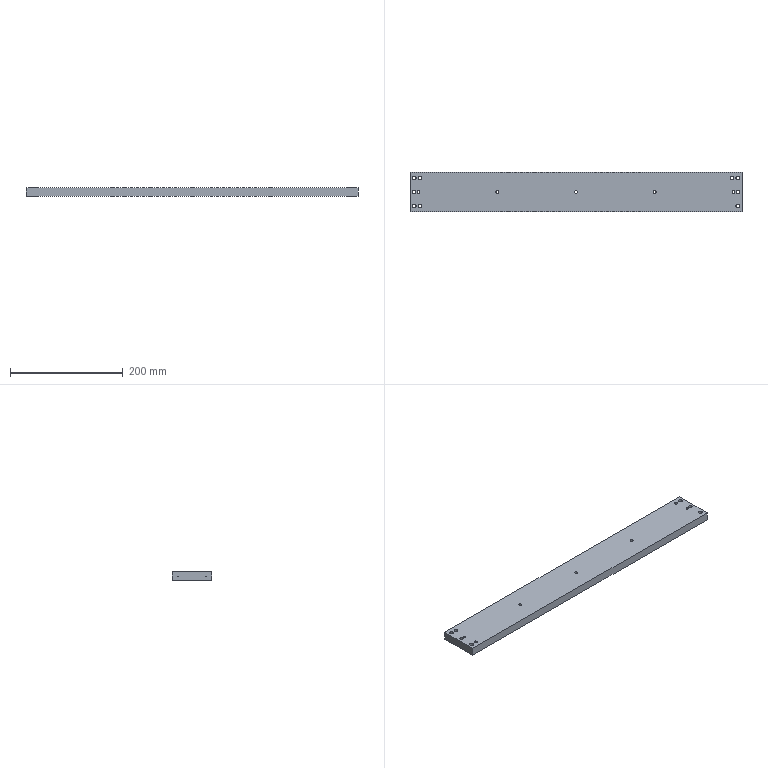Part | NX | 1 solid | 33 faces | box 590 x 70 x 15 mm | volume 612257 mm3 | cylinder 21 | plane 12 | commonest cylinder face diameters 5 x5 6 x5 6.6 x4 11 x4 3.3 x3
STEP:
#1=CARTESIAN_POINT('',(579.9,33.503,3.695));
#2=VERTEX_POINT('',#1);
#3=CARTESIAN_POINT('',(579.9,33.503,2.305));
#4=VERTEX_POINT('',#3);
#5=CARTESIAN_POINT('',(579.9,35.,3.));
#6=DIRECTION('',(1.,0.,0.));
#7=DIRECTION('',(0.,0.,-1.));
#8=AXIS2_PLACEMENT_3D('',#5,#6,#7);
#9=CIRCLE('',#8,1.65);
#10=EDGE_CURVE('',#2,#4,#9,.T.);
#11=ORIENTED_EDGE('',*,*,#10,.F.);
#12=CARTESIAN_POINT('',(579.9,33.503,2.305));
#13=CARTESIAN_POINT('',(580.015,33.304,2.735));
#14=CARTESIAN_POINT('',(580.015,33.304,3.265));
#15=CARTESIAN_POINT('',(579.9,33.503,3.695));
#16=B_SPLINE_CURVE_WITH_KNOTS('',3,(#12,#13,#14,#15),.UNSPECIFIED.,.F.,.F.,(4,4),(0.,0.001444),.UNSPECIFIED.);
#17=EDGE_CURVE('',#4,#2,#16,.T.);
#18=ORIENTED_EDGE('',*,*,#17,.F.);
#19=EDGE_LOOP('',(#11,#18));
#20=FACE_BOUND('',#19,.T.);
#21=CARTESIAN_POINT('',(590.,35.,3.));
#22=DIRECTION('',(1.,0.,0.));
#23=DIRECTION('',(0.,0.,-1.));
#24=AXIS2_PLACEMENT_3D('',#21,#22,#23);
#25=CYLINDRICAL_SURFACE('',#24,1.65);
#26=ADVANCED_FACE('',(#20),#25,.F.);
#27=ORIENTED_EDGE('',*,*,#10,.T.);
#28=CARTESIAN_POINT('',(579.9,33.503,0.));
#29=DIRECTION('',(0.,0.,-1.));
#30=VECTOR('',#29,1000.);
#31=LINE('',#28,#30);
#32=EDGE_CURVE('',#2,#4,#31,.T.);
#33=ORIENTED_EDGE('',*,*,#32,.F.);
#34=EDGE_LOOP('',(#27,#33));
#35=FACE_BOUND('',#34,.T.);
#36=CARTESIAN_POINT('',(579.9,35.,3.));
#37=DIRECTION('',(-1.,0.,0.));
#38=DIRECTION('',(0.,0.,1.));
#39=AXIS2_PLACEMENT_3D('',#36,#37,#38);
#40=PLANE('',#39);
#41=ADVANCED_FACE('',(#35),#40,.F.);
#42=CARTESIAN_POINT('',(579.9,36.497,2.305));
#43=VERTEX_POINT('',#42);
#44=CARTESIAN_POINT('',(579.9,36.497,3.695));
#45=VERTEX_POINT('',#44);
#46=CARTESIAN_POINT('',(579.9,35.,3.));
#47=DIRECTION('',(1.,0.,0.));
#48=DIRECTION('',(0.,0.,-1.));
#49=AXIS2_PLACEMENT_3D('',#46,#47,#48);
#50=CIRCLE('',#49,1.65);
#51=EDGE_CURVE('',#43,#45,#50,.T.);
#52=ORIENTED_EDGE('',*,*,#51,.T.);
#53=CARTESIAN_POINT('',(579.9,36.497,0.));
#54=DIRECTION('',(0.,0.,1.));
#55=VECTOR('',#54,1000.);
#56=LINE('',#53,#55);
#57=EDGE_CURVE('',#43,#45,#56,.T.);
#58=ORIENTED_EDGE('',*,*,#57,.F.);
#59=EDGE_LOOP('',(#52,#58));
#60=FACE_BOUND('',#59,.T.);
#61=CARTESIAN_POINT('',(579.9,35.,3.));
#62=DIRECTION('',(-1.,0.,0.));
#63=DIRECTION('',(0.,0.,1.));
#64=AXIS2_PLACEMENT_3D('',#61,#62,#63);
#65=PLANE('',#64);
#66=ADVANCED_FACE('',(#60),#65,.F.);
#67=ORIENTED_EDGE('',*,*,#51,.F.);
#68=CARTESIAN_POINT('',(579.9,36.497,3.695));
#69=CARTESIAN_POINT('',(580.015,36.696,3.265));
#70=CARTESIAN_POINT('',(580.015,36.696,2.735));
#71=CARTESIAN_POINT('',(579.9,36.497,2.305));
#72=B_SPLINE_CURVE_WITH_KNOTS('',3,(#68,#69,#70,#71),.UNSPECIFIED.,.F.,.F.,(4,4),(0.,0.001444),.UNSPECIFIED.);
#73=EDGE_CURVE('',#45,#43,#72,.T.);
#74=ORIENTED_EDGE('',*,*,#73,.F.);
#75=EDGE_LOOP('',(#67,#74));
#76=FACE_BOUND('',#75,.T.);
#77=CARTESIAN_POINT('',(590.,35.,3.));
#78=DIRECTION('',(1.,0.,0.));
#79=DIRECTION('',(0.,0.,-1.));
#80=AXIS2_PLACEMENT_3D('',#77,#78,#79);
#81=CYLINDRICAL_SURFACE('',#80,1.65);
#82=ADVANCED_FACE('',(#76),#81,.F.);
#83=CARTESIAN_POINT('',(2.,10.,6.4));
#84=VERTEX_POINT('',#83);
#85=CARTESIAN_POINT('',(7.5,10.,6.4));
#86=DIRECTION('',(0.,0.,-1.));
#87=DIRECTION('',(-1.,0.,0.));
#88=AXIS2_PLACEMENT_3D('',#85,#86,#87);
#89=CIRCLE('',#88,5.5);
#90=EDGE_CURVE('',#84,#84,#89,.T.);
#91=ORIENTED_EDGE('',*,*,#90,.T.);
#92=EDGE_LOOP('',(#91));
#93=FACE_BOUND('',#92,.T.);
#94=CARTESIAN_POINT('',(4.2,10.,6.4));
#95=VERTEX_POINT('',#94);
#96=CARTESIAN_POINT('',(7.5,10.,6.4));
#97=DIRECTION('',(0.,0.,-1.));
#98=DIRECTION('',(-1.,0.,0.));
#99=AXIS2_PLACEMENT_3D('',#96,#97,#98);
#100=CIRCLE('',#99,3.3);
#101=EDGE_CURVE('',#95,#95,#100,.T.);
#102=ORIENTED_EDGE('',*,*,#101,.F.);
#103=EDGE_LOOP('',(#102));
#104=FACE_BOUND('',#103,.T.);
#105=CARTESIAN_POINT('',(10.8,10.,6.4));
#106=DIRECTION('',(0.,0.,1.));
#107=DIRECTION('',(1.,0.,0.));
#108=AXIS2_PLACEMENT_3D('',#105,#106,#107);
#109=PLANE('',#108);
#110=ADVANCED_FACE('',(#93,#104),#109,.F.);
#111=CARTESIAN_POINT('',(13.,60.,6.4));
#112=VERTEX_POINT('',#111);
#113=CARTESIAN_POINT('',(7.5,60.,6.4));
#114=DIRECTION('',(0.,0.,-1.));
#115=DIRECTION('',(1.,0.,0.));
#116=AXIS2_PLACEMENT_3D('',#113,#114,#115);
#117=CIRCLE('',#116,5.5);
#118=EDGE_CURVE('',#112,#112,#117,.T.);
#119=ORIENTED_EDGE('',*,*,#118,.T.);
#120=EDGE_LOOP('',(#119));
#121=FACE_BOUND('',#120,.T.);
#122=CARTESIAN_POINT('',(10.8,60.,6.4));
#123=VERTEX_POINT('',#122);
#124=CARTESIAN_POINT('',(7.5,60.,6.4));
#125=DIRECTION('',(0.,0.,-1.));
#126=DIRECTION('',(1.,0.,0.));
#127=AXIS2_PLACEMENT_3D('',#124,#125,#126);
#128=CIRCLE('',#127,3.3);
#129=EDGE_CURVE('',#123,#123,#128,.T.);
#130=ORIENTED_EDGE('',*,*,#129,.F.);
#131=EDGE_LOOP('',(#130));
#132=FACE_BOUND('',#131,.T.);
#133=CARTESIAN_POINT('',(10.8,10.,6.4));
#134=DIRECTION('',(0.,0.,1.));
#135=DIRECTION('',(1.,0.,0.));
#136=AXIS2_PLACEMENT_3D('',#133,#134,#135);
#137=PLANE('',#136);
#138=ADVANCED_FACE('',(#121,#132),#137,.F.);
#139=CARTESIAN_POINT('',(588.,10.,6.4));
#140=VERTEX_POINT('',#139);
#141=CARTESIAN_POINT('',(582.5,10.,6.4));
#142=DIRECTION('',(0.,0.,-1.));
#143=DIRECTION('',(1.,0.,0.));
#144=AXIS2_PLACEMENT_3D('',#141,#142,#143);
#145=CIRCLE('',#144,5.5);
#146=EDGE_CURVE('',#140,#140,#145,.T.);
#147=ORIENTED_EDGE('',*,*,#146,.T.);
#148=EDGE_LOOP('',(#147));
#149=FACE_BOUND('',#148,.T.);
#150=CARTESIAN_POINT('',(585.8,10.,6.4));
#151=VERTEX_POINT('',#150);
#152=CARTESIAN_POINT('',(582.5,10.,6.4));
#153=DIRECTION('',(0.,0.,-1.));
#154=DIRECTION('',(1.,0.,0.));
#155=AXIS2_PLACEMENT_3D('',#152,#153,#154);
#156=CIRCLE('',#155,3.3);
#157=EDGE_CURVE('',#151,#151,#156,.T.);
#158=ORIENTED_EDGE('',*,*,#157,.F.);
#159=EDGE_LOOP('',(#158));
#160=FACE_BOUND('',#159,.T.);
#161=CARTESIAN_POINT('',(10.8,10.,6.4));
#162=DIRECTION('',(0.,0.,1.));
#163=DIRECTION('',(1.,0.,0.));
#164=AXIS2_PLACEMENT_3D('',#161,#162,#163);
#165=PLANE('',#164);
#166=ADVANCED_FACE('',(#149,#160),#165,.F.);
#167=CARTESIAN_POINT('',(588.,60.,6.4));
#168=VERTEX_POINT('',#167);
#169=CARTESIAN_POINT('',(582.5,60.,6.4));
#170=DIRECTION('',(0.,0.,-1.));
#171=DIRECTION('',(1.,0.,0.));
#172=AXIS2_PLACEMENT_3D('',#169,#170,#171);
#173=CIRCLE('',#172,5.5);
#174=EDGE_CURVE('',#168,#168,#173,.T.);
#175=ORIENTED_EDGE('',*,*,#174,.T.);
#176=EDGE_LOOP('',(#175));
#177=FACE_BOUND('',#176,.T.);
#178=CARTESIAN_POINT('',(585.8,60.,6.4));
#179=VERTEX_POINT('',#178);
#180=CARTESIAN_POINT('',(582.5,60.,6.4));
#181=DIRECTION('',(0.,0.,-1.));
#182=DIRECTION('',(1.,0.,0.));
#183=AXIS2_PLACEMENT_3D('',#180,#181,#182);
#184=CIRCLE('',#183,3.3);
#185=EDGE_CURVE('',#179,#179,#184,.T.);
#186=ORIENTED_EDGE('',*,*,#185,.F.);
#187=EDGE_LOOP('',(#186));
#188=FACE_BOUND('',#187,.T.);
#189=CARTESIAN_POINT('',(10.8,10.,6.4));
#190=DIRECTION('',(0.,0.,1.));
#191=DIRECTION('',(1.,0.,0.));
#192=AXIS2_PLACEMENT_3D('',#189,#190,#191);
#193=PLANE('',#192);
#194=ADVANCED_FACE('',(#177,#188),#193,.F.);
#195=CARTESIAN_POINT('',(0.,70.,0.));
#196=VERTEX_POINT('',#195);
#197=CARTESIAN_POINT('',(0.,0.,0.));
#198=VERTEX_POINT('',#197);
#199=CARTESIAN_POINT('',(0.,0.,0.));
#200=DIRECTION('',(0.,-1.,0.));
#201=VECTOR('',#200,1000.);
#202=LINE('',#199,#201);
#203=EDGE_CURVE('',#196,#198,#202,.T.);
#204=ORIENTED_EDGE('',*,*,#203,.F.);
#205=CARTESIAN_POINT('',(590.,70.,0.));
#206=VERTEX_POINT('',#205);
#207=CARTESIAN_POINT('',(0.,70.,0.));
#208=DIRECTION('',(-1.,0.,0.));
#209=VECTOR('',#208,1000.);
#210=LINE('',#207,#209);
#211=EDGE_CURVE('',#206,#196,#210,.T.);
#212=ORIENTED_EDGE('',*,*,#211,.F.);
#213=CARTESIAN_POINT('',(590.,0.,0.));
#214=VERTEX_POINT('',#213);
#215=CARTESIAN_POINT('',(590.,0.,0.));
#216=DIRECTION('',(0.,1.,0.));
#217=VECTOR('',#216,1000.);
#218=LINE('',#215,#217);
#219=EDGE_CURVE('',#214,#206,#218,.T.);
#220=ORIENTED_EDGE('',*,*,#219,.F.);
#221=CARTESIAN_POINT('',(0.,0.,0.));
#222=DIRECTION('',(1.,0.,0.));
#223=VECTOR('',#222,1000.);
#224=LINE('',#221,#223);
#225=EDGE_CURVE('',#198,#214,#224,.T.);
#226=ORIENTED_EDGE('',*,*,#225,.F.);
#227=EDGE_LOOP('',(#204,#212,#220,#226));
#228=FACE_BOUND('',#227,.T.);
#229=CARTESIAN_POINT('',(577.,60.,0.));
#230=VERTEX_POINT('',#229);
#231=CARTESIAN_POINT('',(582.5,60.,0.));
#232=DIRECTION('',(0.,0.,-1.));
#233=DIRECTION('',(-1.,0.,0.));
#234=AXIS2_PLACEMENT_3D('',#231,#232,#233);
#235=CIRCLE('',#234,5.5);
#236=EDGE_CURVE('',#230,#230,#235,.T.);
#237=ORIENTED_EDGE('',*,*,#236,.F.);
#238=EDGE_LOOP('',(#237));
#239=FACE_BOUND('',#238,.T.);
#240=CARTESIAN_POINT('',(577.,10.,0.));
#241=VERTEX_POINT('',#240);
#242=CARTESIAN_POINT('',(582.5,10.,0.));
#243=DIRECTION('',(0.,0.,-1.));
#244=DIRECTION('',(-1.,0.,0.));
#245=AXIS2_PLACEMENT_3D('',#242,#243,#244);
#246=CIRCLE('',#245,5.5);
#247=EDGE_CURVE('',#241,#241,#246,.T.);
#248=ORIENTED_EDGE('',*,*,#247,.F.);
#249=EDGE_LOOP('',(#248));
#250=FACE_BOUND('',#249,.T.);
#251=CARTESIAN_POINT('',(2.,60.,0.));
#252=VERTEX_POINT('',#251);
#253=CARTESIAN_POINT('',(7.5,60.,0.));
#254=DIRECTION('',(0.,0.,-1.));
#255=DIRECTION('',(-1.,0.,0.));
#256=AXIS2_PLACEMENT_3D('',#253,#254,#255);
#257=CIRCLE('',#256,5.5);
#258=EDGE_CURVE('',#252,#252,#257,.T.);
#259=ORIENTED_EDGE('',*,*,#258,.F.);
#260=EDGE_LOOP('',(#259));
#261=FACE_BOUND('',#260,.T.);
#262=CARTESIAN_POINT('',(2.,10.,0.));
#263=VERTEX_POINT('',#262);
#264=CARTESIAN_POINT('',(7.5,10.,0.));
#265=DIRECTION('',(0.,0.,-1.));
#266=DIRECTION('',(-1.,0.,0.));
#267=AXIS2_PLACEMENT_3D('',#264,#265,#266);
#268=CIRCLE('',#267,5.5);
#269=EDGE_CURVE('',#263,#263,#268,.T.);
#270=ORIENTED_EDGE('',*,*,#269,.F.);
#271=EDGE_LOOP('',(#270));
#272=FACE_BOUND('',#271,.T.);
#273=CARTESIAN_POINT('',(572.5,35.,0.));
#274=VERTEX_POINT('',#273);
#275=CARTESIAN_POINT('',(575.,35.,0.));
#276=DIRECTION('',(0.,0.,-1.));
#277=DIRECTION('',(-1.,0.,0.));
#278=AXIS2_PLACEMENT_3D('',#275,#276,#277);
#279=CIRCLE('',#278,2.5);
#280=EDGE_CURVE('',#274,#274,#279,.T.);
#281=ORIENTED_EDGE('',*,*,#280,.F.);
#282=EDGE_LOOP('',(#281));
#283=FACE_BOUND('',#282,.T.);
#284=CARTESIAN_POINT('',(432.5,35.,0.));
#285=VERTEX_POINT('',#284);
#286=CARTESIAN_POINT('',(435.,35.,0.));
#287=DIRECTION('',(0.,0.,-1.));
#288=DIRECTION('',(-1.,0.,0.));
#289=AXIS2_PLACEMENT_3D('',#286,#287,#288);
#290=CIRCLE('',#289,2.5);
#291=EDGE_CURVE('',#285,#285,#290,.T.);
#292=ORIENTED_EDGE('',*,*,#291,.F.);
#293=EDGE_LOOP('',(#292));
#294=FACE_BOUND('',#293,.T.);
#295=CARTESIAN_POINT('',(292.5,35.,0.));
#296=VERTEX_POINT('',#295);
#297=CARTESIAN_POINT('',(295.,35.,0.));
#298=DIRECTION('',(0.,0.,-1.));
#299=DIRECTION('',(-1.,0.,0.));
#300=AXIS2_PLACEMENT_3D('',#297,#298,#299);
#301=CIRCLE('',#300,2.5);
#302=EDGE_CURVE('',#296,#296,#301,.T.);
#303=ORIENTED_EDGE('',*,*,#302,.F.);
#304=EDGE_LOOP('',(#303));
#305=FACE_BOUND('',#304,.T.);
#306=CARTESIAN_POINT('',(152.5,35.,0.));
#307=VERTEX_POINT('',#306);
#308=CARTESIAN_POINT('',(155.,35.,0.));
#309=DIRECTION('',(0.,0.,-1.));
#310=DIRECTION('',(-1.,0.,0.));
#311=AXIS2_PLACEMENT_3D('',#308,#309,#310);
#312=CIRCLE('',#311,2.5);
#313=EDGE_CURVE('',#307,#307,#312,.T.);
#314=ORIENTED_EDGE('',*,*,#313,.F.);
#315=EDGE_LOOP('',(#314));
#316=FACE_BOUND('',#315,.T.);
#317=CARTESIAN_POINT('',(12.5,35.,0.));
#318=VERTEX_POINT('',#317);
#319=CARTESIAN_POINT('',(15.,35.,0.));
#320=DIRECTION('',(0.,0.,-1.));
#321=DIRECTION('',(-1.,0.,0.));
#322=AXIS2_PLACEMENT_3D('',#319,#320,#321);
#323=CIRCLE('',#322,2.5);
#324=EDGE_CURVE('',#318,#318,#323,.T.);
#325=ORIENTED_EDGE('',*,*,#324,.F.);
#326=EDGE_LOOP('',(#325));
#327=FACE_BOUND('',#326,.T.);
#328=CARTESIAN_POINT('',(569.,60.,0.));
#329=VERTEX_POINT('',#328);
#330=CARTESIAN_POINT('',(572.,60.,0.));
#331=DIRECTION('',(0.,0.,-1.));
#332=DIRECTION('',(-1.,0.,0.));
#333=AXIS2_PLACEMENT_3D('',#330,#331,#332);
#334=CIRCLE('',#333,3.);
#335=EDGE_CURVE('',#329,#329,#334,.T.);
#336=ORIENTED_EDGE('',*,*,#335,.F.);
#337=EDGE_LOOP('',(#336));
#338=FACE_BOUND('',#337,.T.);
#339=CARTESIAN_POINT('',(15.,60.,0.));
#340=VERTEX_POINT('',#339);
#341=CARTESIAN_POINT('',(18.,60.,0.));
#342=DIRECTION('',(0.,0.,-1.));
#343=DIRECTION('',(-1.,0.,0.));
#344=AXIS2_PLACEMENT_3D('',#341,#342,#343);
#345=CIRCLE('',#344,3.);
#346=EDGE_CURVE('',#340,#340,#345,.T.);
#347=ORIENTED_EDGE('',*,*,#346,.F.);
#348=EDGE_LOOP('',(#347));
#349=FACE_BOUND('',#348,.T.);
#350=CARTESIAN_POINT('',(15.,10.,0.));
#351=VERTEX_POINT('',#350);
#352=CARTESIAN_POINT('',(18.,10.,0.));
#353=DIRECTION('',(0.,0.,-1.));
#354=DIRECTION('',(-1.,0.,0.));
#355=AXIS2_PLACEMENT_3D('',#352,#353,#354);
#356=CIRCLE('',#355,3.);
#357=EDGE_CURVE('',#351,#351,#356,.T.);
#358=ORIENTED_EDGE('',*,*,#357,.F.);
#359=EDGE_LOOP('',(#358));
#360=FACE_BOUND('',#359,.T.);
#361=CARTESIAN_POINT('',(579.5,35.,0.));
#362=VERTEX_POINT('',#361);
#363=CARTESIAN_POINT('',(582.5,35.,0.));
#364=DIRECTION('',(0.,0.,-1.));
#365=DIRECTION('',(-1.,0.,0.));
#366=AXIS2_PLACEMENT_3D('',#363,#364,#365);
#367=CIRCLE('',#366,3.);
#368=EDGE_CURVE('',#362,#362,#367,.T.);
#369=ORIENTED_EDGE('',*,*,#368,.F.);
#370=EDGE_LOOP('',(#369));
#371=FACE_BOUND('',#370,.T.);
#372=CARTESIAN_POINT('',(4.5,35.,0.));
#373=VERTEX_POINT('',#372);
#374=CARTESIAN_POINT('',(7.5,35.,0.));
#375=DIRECTION('',(0.,0.,-1.));
#376=DIRECTION('',(-1.,0.,0.));
#377=AXIS2_PLACEMENT_3D('',#374,#375,#376);
#378=CIRCLE('',#377,3.);
#379=EDGE_CURVE('',#373,#373,#378,.T.);
#380=ORIENTED_EDGE('',*,*,#379,.F.);
#381=EDGE_LOOP('',(#380));
#382=FACE_BOUND('',#381,.T.);
#383=CARTESIAN_POINT('',(0.,0.,0.));
#384=DIRECTION('',(0.,0.,-1.));
#385=DIRECTION('',(-1.,0.,0.));
#386=AXIS2_PLACEMENT_3D('',#383,#384,#385);
#387=PLANE('',#386);
#388=ADVANCED_FACE('',(#228,#239,#250,#261,#272,#283,#294,#305,#316,#327,#338,#349,#360,#371,#382),#387,.T.);
#389=CARTESIAN_POINT('',(0.,70.,15.));
#390=VERTEX_POINT('',#389);
#391=CARTESIAN_POINT('',(0.,0.,15.));
#392=VERTEX_POINT('',#391);
#393=CARTESIAN_POINT('',(0.,0.,15.));
#394=DIRECTION('',(0.,-1.,0.));
#395=VECTOR('',#394,1000.);
#396=LINE('',#393,#395);
#397=EDGE_CURVE('',#390,#392,#396,.T.);
#398=ORIENTED_EDGE('',*,*,#397,.T.);
#399=CARTESIAN_POINT('',(590.,0.,15.));
#400=VERTEX_POINT('',#399);
#401=CARTESIAN_POINT('',(0.,0.,15.));
#402=DIRECTION('',(1.,0.,0.));
#403=VECTOR('',#402,1000.);
#404=LINE('',#401,#403);
#405=EDGE_CURVE('',#392,#400,#404,.T.);
#406=ORIENTED_EDGE('',*,*,#405,.T.);
#407=CARTESIAN_POINT('',(590.,70.,15.));
#408=VERTEX_POINT('',#407);
#409=CARTESIAN_POINT('',(590.,0.,15.));
#410=DIRECTION('',(0.,1.,0.));
#411=VECTOR('',#410,1000.);
#412=LINE('',#409,#411);
#413=EDGE_CURVE('',#400,#408,#412,.T.);
#414=ORIENTED_EDGE('',*,*,#413,.T.);
#415=CARTESIAN_POINT('',(0.,70.,15.));
#416=DIRECTION('',(-1.,0.,0.));
#417=VECTOR('',#416,1000.);
#418=LINE('',#415,#417);
#419=EDGE_CURVE('',#408,#390,#418,.T.);
#420=ORIENTED_EDGE('',*,*,#419,.T.);
#421=EDGE_LOOP('',(#398,#406,#414,#420));
#422=FACE_BOUND('',#421,.T.);
#423=CARTESIAN_POINT('',(579.2,60.,15.));
#424=VERTEX_POINT('',#423);
#425=CARTESIAN_POINT('',(582.5,60.,15.));
#426=DIRECTION('',(0.,0.,-1.));
#427=DIRECTION('',(-1.,0.,0.));
#428=AXIS2_PLACEMENT_3D('',#425,#426,#427);
#429=CIRCLE('',#428,3.3);
#430=EDGE_CURVE('',#424,#424,#429,.T.);
#431=ORIENTED_EDGE('',*,*,#430,.T.);
#432=EDGE_LOOP('',(#431));
#433=FACE_BOUND('',#432,.T.);
#434=CARTESIAN_POINT('',(579.2,10.,15.));
#435=VERTEX_POINT('',#434);
#436=CARTESIAN_POINT('',(582.5,10.,15.));
#437=DIRECTION('',(0.,0.,-1.));
#438=DIRECTION('',(-1.,0.,0.));
#439=AXIS2_PLACEMENT_3D('',#436,#437,#438);
#440=CIRCLE('',#439,3.3);
#441=EDGE_CURVE('',#435,#435,#440,.T.);
#442=ORIENTED_EDGE('',*,*,#441,.T.);
#443=EDGE_LOOP('',(#442));
#444=FACE_BOUND('',#443,.T.);
#445=CARTESIAN_POINT('',(4.2,60.,15.));
#446=VERTEX_POINT('',#445);
#447=CARTESIAN_POINT('',(7.5,60.,15.));
#448=DIRECTION('',(0.,0.,-1.));
#449=DIRECTION('',(-1.,0.,0.));
#450=AXIS2_PLACEMENT_3D('',#447,#448,#449);
#451=CIRCLE('',#450,3.3);
#452=EDGE_CURVE('',#446,#446,#451,.T.);
#453=ORIENTED_EDGE('',*,*,#452,.T.);
#454=EDGE_LOOP('',(#453));
#455=FACE_BOUND('',#454,.T.);
#456=CARTESIAN_POINT('',(4.2,10.,15.));
#457=VERTEX_POINT('',#456);
#458=CARTESIAN_POINT('',(7.5,10.,15.));
#459=DIRECTION('',(0.,0.,-1.));
#460=DIRECTION('',(-1.,0.,0.));
#461=AXIS2_PLACEMENT_3D('',#458,#459,#460);
#462=CIRCLE('',#461,3.3);
#463=EDGE_CURVE('',#457,#457,#462,.T.);
#464=ORIENTED_EDGE('',*,*,#463,.T.);
#465=EDGE_LOOP('',(#464));
#466=FACE_BOUND('',#465,.T.);
#467=CARTESIAN_POINT('',(572.5,35.,15.));
#468=VERTEX_POINT('',#467);
#469=CARTESIAN_POINT('',(575.,35.,15.));
#470=DIRECTION('',(0.,0.,-1.));
#471=DIRECTION('',(-1.,0.,0.));
#472=AXIS2_PLACEMENT_3D('',#469,#470,#471);
#473=CIRCLE('',#472,2.5);
#474=EDGE_CURVE('',#468,#468,#473,.T.);
#475=ORIENTED_EDGE('',*,*,#474,.T.);
#476=EDGE_LOOP('',(#475));
#477=FACE_BOUND('',#476,.T.);
#478=CARTESIAN_POINT('',(432.5,35.,15.));
#479=VERTEX_POINT('',#478);
#480=CARTESIAN_POINT('',(435.,35.,15.));
#481=DIRECTION('',(0.,0.,-1.));
#482=DIRECTION('',(-1.,0.,0.));
#483=AXIS2_PLACEMENT_3D('',#480,#481,#482);
#484=CIRCLE('',#483,2.5);
#485=EDGE_CURVE('',#479,#479,#484,.T.);
#486=ORIENTED_EDGE('',*,*,#485,.T.);
#487=EDGE_LOOP('',(#486));
#488=FACE_BOUND('',#487,.T.);
#489=CARTESIAN_POINT('',(292.5,35.,15.));
#490=VERTEX_POINT('',#489);
#491=CARTESIAN_POINT('',(295.,35.,15.));
#492=DIRECTION('',(0.,0.,-1.));
#493=DIRECTION('',(-1.,0.,0.));
#494=AXIS2_PLACEMENT_3D('',#491,#492,#493);
#495=CIRCLE('',#494,2.5);
#496=EDGE_CURVE('',#490,#490,#495,.T.);
#497=ORIENTED_EDGE('',*,*,#496,.T.);
#498=EDGE_LOOP('',(#497));
#499=FACE_BOUND('',#498,.T.);
#500=CARTESIAN_POINT('',(152.5,35.,15.));
#501=VERTEX_POINT('',#500);
#502=CARTESIAN_POINT('',(155.,35.,15.));
#503=DIRECTION('',(0.,0.,-1.));
#504=DIRECTION('',(-1.,0.,0.));
#505=AXIS2_PLACEMENT_3D('',#502,#503,#504);
#506=CIRCLE('',#505,2.5);
#507=EDGE_CURVE('',#501,#501,#506,.T.);
#508=ORIENTED_EDGE('',*,*,#507,.T.);
#509=EDGE_LOOP('',(#508));
#510=FACE_BOUND('',#509,.T.);
#511=CARTESIAN_POINT('',(12.5,35.,15.));
#512=VERTEX_POINT('',#511);
#513=CARTESIAN_POINT('',(15.,35.,15.));
#514=DIRECTION('',(0.,0.,-1.));
#515=DIRECTION('',(-1.,0.,0.));
#516=AXIS2_PLACEMENT_3D('',#513,#514,#515);
#517=CIRCLE('',#516,2.5);
#518=EDGE_CURVE('',#512,#512,#517,.T.);
#519=ORIENTED_EDGE('',*,*,#518,.T.);
#520=EDGE_LOOP('',(#519));
#521=FACE_BOUND('',#520,.T.);
#522=CARTESIAN_POINT('',(569.,60.,15.));
#523=VERTEX_POINT('',#522);
#524=CARTESIAN_POINT('',(572.,60.,15.));
#525=DIRECTION('',(0.,0.,-1.));
#526=DIRECTION('',(-1.,0.,0.));
#527=AXIS2_PLACEMENT_3D('',#524,#525,#526);
#528=CIRCLE('',#527,3.);
#529=EDGE_CURVE('',#523,#523,#528,.T.);
#530=ORIENTED_EDGE('',*,*,#529,.T.);
#531=EDGE_LOOP('',(#530));
#532=FACE_BOUND('',#531,.T.);
#533=CARTESIAN_POINT('',(15.,60.,15.));
#534=VERTEX_POINT('',#533);
#535=CARTESIAN_POINT('',(18.,60.,15.));
#536=DIRECTION('',(0.,0.,-1.));
#537=DIRECTION('',(-1.,0.,0.));
#538=AXIS2_PLACEMENT_3D('',#535,#536,#537);
#539=CIRCLE('',#538,3.);
#540=EDGE_CURVE('',#534,#534,#539,.T.);
#541=ORIENTED_EDGE('',*,*,#540,.T.);
#542=EDGE_LOOP('',(#541));
#543=FACE_BOUND('',#542,.T.);
#544=CARTESIAN_POINT('',(15.,10.,15.));
#545=VERTEX_POINT('',#544);
#546=CARTESIAN_POINT('',(18.,10.,15.));
#547=DIRECTION('',(0.,0.,-1.));
#548=DIRECTION('',(-1.,0.,0.));
#549=AXIS2_PLACEMENT_3D('',#546,#547,#548);
#550=CIRCLE('',#549,3.);
#551=EDGE_CURVE('',#545,#545,#550,.T.);
#552=ORIENTED_EDGE('',*,*,#551,.T.);
#553=EDGE_LOOP('',(#552));
#554=FACE_BOUND('',#553,.T.);
#555=CARTESIAN_POINT('',(579.5,35.,15.));
#556=VERTEX_POINT('',#555);
#557=CARTESIAN_POINT('',(582.5,35.,15.));
#558=DIRECTION('',(0.,0.,-1.));
#559=DIRECTION('',(-1.,0.,0.));
#560=AXIS2_PLACEMENT_3D('',#557,#558,#559);
#561=CIRCLE('',#560,3.);
#562=EDGE_CURVE('',#556,#556,#561,.T.);
#563=ORIENTED_EDGE('',*,*,#562,.T.);
#564=EDGE_LOOP('',(#563));
#565=FACE_BOUND('',#564,.T.);
#566=CARTESIAN_POINT('',(4.5,35.,15.));
#567=VERTEX_POINT('',#566);
#568=CARTESIAN_POINT('',(7.5,35.,15.));
#569=DIRECTION('',(0.,0.,-1.));
#570=DIRECTION('',(-1.,0.,0.));
#571=AXIS2_PLACEMENT_3D('',#568,#569,#570);
#572=CIRCLE('',#571,3.);
#573=EDGE_CURVE('',#567,#567,#572,.T.);
#574=ORIENTED_EDGE('',*,*,#573,.T.);
#575=EDGE_LOOP('',(#574));
#576=FACE_BOUND('',#575,.T.);
#577=CARTESIAN_POINT('',(0.,0.,15.));
#578=DIRECTION('',(0.,0.,-1.));
#579=DIRECTION('',(-1.,0.,0.));
#580=AXIS2_PLACEMENT_3D('',#577,#578,#579);
#581=PLANE('',#580);
#582=ADVANCED_FACE('',(#422,#433,#444,#455,#466,#477,#488,#499,#510,#521,#532,#543,#554,#565,#576),#581,.F.);
#583=ORIENTED_EDGE('',*,*,#211,.T.);
#584=CARTESIAN_POINT('',(0.,70.,15.));
#585=DIRECTION('',(0.,0.,-1.));
#586=VECTOR('',#585,1000.);
#587=LINE('',#584,#586);
#588=EDGE_CURVE('',#390,#196,#587,.T.);
#589=ORIENTED_EDGE('',*,*,#588,.F.);
#590=ORIENTED_EDGE('',*,*,#419,.F.);
#591=CARTESIAN_POINT('',(590.,70.,15.));
#592=DIRECTION('',(0.,0.,-1.));
#593=VECTOR('',#592,1000.);
#594=LINE('',#591,#593);
#595=EDGE_CURVE('',#408,#206,#594,.T.);
#596=ORIENTED_EDGE('',*,*,#595,.T.);
#597=EDGE_LOOP('',(#583,#589,#590,#596));
#598=FACE_BOUND('',#597,.T.);
#599=CARTESIAN_POINT('',(0.,70.,15.));
#600=DIRECTION('',(0.,-1.,0.));
#601=DIRECTION('',(0.,0.,-1.));
#602=AXIS2_PLACEMENT_3D('',#599,#600,#601);
#603=PLANE('',#602);
#604=ADVANCED_FACE('',(#598),#603,.F.);
#605=ORIENTED_EDGE('',*,*,#219,.T.);
#606=ORIENTED_EDGE('',*,*,#595,.F.);
#607=ORIENTED_EDGE('',*,*,#413,.F.);
#608=CARTESIAN_POINT('',(590.,0.,15.));
#609=DIRECTION('',(0.,0.,-1.));
#610=VECTOR('',#609,1000.);
#611=LINE('',#608,#610);
#612=EDGE_CURVE('',#400,#214,#611,.T.);
#613=ORIENTED_EDGE('',*,*,#612,.T.);
#614=EDGE_LOOP('',(#605,#606,#607,#613));
#615=FACE_BOUND('',#614,.T.);
#616=CARTESIAN_POINT('',(590.,35.,1.35));
#617=VERTEX_POINT('',#616);
#618=CARTESIAN_POINT('',(590.,35.,3.));
#619=DIRECTION('',(1.,0.,0.));
#620=DIRECTION('',(0.,0.,-1.));
#621=AXIS2_PLACEMENT_3D('',#618,#619,#620);
#622=CIRCLE('',#621,1.65);
#623=EDGE_CURVE('',#617,#617,#622,.T.);
#624=ORIENTED_EDGE('',*,*,#623,.F.);
#625=EDGE_LOOP('',(#624));
#626=FACE_BOUND('',#625,.T.);
#627=CARTESIAN_POINT('',(590.,0.,15.));
#628=DIRECTION('',(-1.,0.,0.));
#629=DIRECTION('',(0.,0.,1.));
#630=AXIS2_PLACEMENT_3D('',#627,#628,#629);
#631=PLANE('',#630);
#632=ADVANCED_FACE('',(#615,#626),#631,.F.);
#633=ORIENTED_EDGE('',*,*,#225,.T.);
#634=ORIENTED_EDGE('',*,*,#612,.F.);
#635=ORIENTED_EDGE('',*,*,#405,.F.);
#636=CARTESIAN_POINT('',(0.,0.,15.));
#637=DIRECTION('',(0.,0.,-1.));
#638=VECTOR('',#637,1000.);
#639=LINE('',#636,#638);
#640=EDGE_CURVE('',#392,#198,#639,.T.);
#641=ORIENTED_EDGE('',*,*,#640,.T.);
#642=EDGE_LOOP('',(#633,#634,#635,#641));
#643=FACE_BOUND('',#642,.T.);
#644=CARTESIAN_POINT('',(0.,0.,15.));
#645=DIRECTION('',(0.,1.,0.));
#646=DIRECTION('',(0.,0.,1.));
#647=AXIS2_PLACEMENT_3D('',#644,#645,#646);
#648=PLANE('',#647);
#649=ADVANCED_FACE('',(#643),#648,.F.);
#650=ORIENTED_EDGE('',*,*,#203,.T.);
#651=ORIENTED_EDGE('',*,*,#640,.F.);
#652=ORIENTED_EDGE('',*,*,#397,.F.);
#653=ORIENTED_EDGE('',*,*,#588,.T.);
#654=EDGE_LOOP('',(#650,#651,#652,#653));
#655=FACE_BOUND('',#654,.T.);
#656=CARTESIAN_POINT('',(0.,0.,15.));
#657=DIRECTION('',(1.,0.,0.));
#658=DIRECTION('',(0.,0.,-1.));
#659=AXIS2_PLACEMENT_3D('',#656,#657,#658);
#660=PLANE('',#659);
#661=ADVANCED_FACE('',(#655),#660,.F.);
#662=ORIENTED_EDGE('',*,*,#185,.T.);
#663=EDGE_LOOP('',(#662));
#664=FACE_BOUND('',#663,.T.);
#665=ORIENTED_EDGE('',*,*,#430,.F.);
#666=EDGE_LOOP('',(#665));
#667=FACE_BOUND('',#666,.T.);
#668=CARTESIAN_POINT('',(582.5,60.,0.));
#669=DIRECTION('',(0.,0.,-1.));
#670=DIRECTION('',(-1.,0.,0.));
#671=AXIS2_PLACEMENT_3D('',#668,#669,#670);
#672=CYLINDRICAL_SURFACE('',#671,3.3);
#673=ADVANCED_FACE('',(#664,#667),#672,.F.);
#674=ORIENTED_EDGE('',*,*,#236,.T.);
#675=EDGE_LOOP('',(#674));
#676=FACE_BOUND('',#675,.T.);
#677=ORIENTED_EDGE('',*,*,#174,.F.);
#678=EDGE_LOOP('',(#677));
#679=FACE_BOUND('',#678,.T.);
#680=CARTESIAN_POINT('',(582.5,60.,0.));
#681=DIRECTION('',(0.,0.,-1.));
#682=DIRECTION('',(-1.,0.,0.));
#683=AXIS2_PLACEMENT_3D('',#680,#681,#682);
#684=CYLINDRICAL_SURFACE('',#683,5.5);
#685=ADVANCED_FACE('',(#676,#679),#684,.F.);
#686=ORIENTED_EDGE('',*,*,#157,.T.);
#687=EDGE_LOOP('',(#686));
#688=FACE_BOUND('',#687,.T.);
#689=ORIENTED_EDGE('',*,*,#441,.F.);
#690=EDGE_LOOP('',(#689));
#691=FACE_BOUND('',#690,.T.);
#692=CARTESIAN_POINT('',(582.5,10.,0.));
#693=DIRECTION('',(0.,0.,-1.));
#694=DIRECTION('',(-1.,0.,0.));
#695=AXIS2_PLACEMENT_3D('',#692,#693,#694);
#696=CYLINDRICAL_SURFACE('',#695,3.3);
#697=ADVANCED_FACE('',(#688,#691),#696,.F.);
#698=ORIENTED_EDGE('',*,*,#247,.T.);
#699=EDGE_LOOP('',(#698));
#700=FACE_BOUND('',#699,.T.);
#701=ORIENTED_EDGE('',*,*,#146,.F.);
#702=EDGE_LOOP('',(#701));
#703=FACE_BOUND('',#702,.T.);
#704=CARTESIAN_POINT('',(582.5,10.,0.));
#705=DIRECTION('',(0.,0.,-1.));
#706=DIRECTION('',(-1.,0.,0.));
#707=AXIS2_PLACEMENT_3D('',#704,#705,#706);
#708=CYLINDRICAL_SURFACE('',#707,5.5);
#709=ADVANCED_FACE('',(#700,#703),#708,.F.);
#710=ORIENTED_EDGE('',*,*,#129,.T.);
#711=EDGE_LOOP('',(#710));
#712=FACE_BOUND('',#711,.T.);
#713=ORIENTED_EDGE('',*,*,#452,.F.);
#714=EDGE_LOOP('',(#713));
#715=FACE_BOUND('',#714,.T.);
#716=CARTESIAN_POINT('',(7.5,60.,0.));
#717=DIRECTION('',(0.,0.,-1.));
#718=DIRECTION('',(-1.,0.,0.));
#719=AXIS2_PLACEMENT_3D('',#716,#717,#718);
#720=CYLINDRICAL_SURFACE('',#719,3.3);
#721=ADVANCED_FACE('',(#712,#715),#720,.F.);
#722=ORIENTED_EDGE('',*,*,#258,.T.);
#723=EDGE_LOOP('',(#722));
#724=FACE_BOUND('',#723,.T.);
#725=ORIENTED_EDGE('',*,*,#118,.F.);
#726=EDGE_LOOP('',(#725));
#727=FACE_BOUND('',#726,.T.);
#728=CARTESIAN_POINT('',(7.5,60.,0.));
#729=DIRECTION('',(0.,0.,-1.));
#730=DIRECTION('',(-1.,0.,0.));
#731=AXIS2_PLACEMENT_3D('',#728,#729,#730);
#732=CYLINDRICAL_SURFACE('',#731,5.5);
#733=ADVANCED_FACE('',(#724,#727),#732,.F.);
#734=ORIENTED_EDGE('',*,*,#101,.T.);
#735=EDGE_LOOP('',(#734));
#736=FACE_BOUND('',#735,.T.);
#737=ORIENTED_EDGE('',*,*,#463,.F.);
#738=EDGE_LOOP('',(#737));
#739=FACE_BOUND('',#738,.T.);
#740=CARTESIAN_POINT('',(7.5,10.,0.));
#741=DIRECTION('',(0.,0.,-1.));
#742=DIRECTION('',(-1.,0.,0.));
#743=AXIS2_PLACEMENT_3D('',#740,#741,#742);
#744=CYLINDRICAL_SURFACE('',#743,3.3);
#745=ADVANCED_FACE('',(#736,#739),#744,.F.);
#746=ORIENTED_EDGE('',*,*,#269,.T.);
#747=EDGE_LOOP('',(#746));
#748=FACE_BOUND('',#747,.T.);
#749=ORIENTED_EDGE('',*,*,#90,.F.);
#750=EDGE_LOOP('',(#749));
#751=FACE_BOUND('',#750,.T.);
#752=CARTESIAN_POINT('',(7.5,10.,0.));
#753=DIRECTION('',(0.,0.,-1.));
#754=DIRECTION('',(-1.,0.,0.));
#755=AXIS2_PLACEMENT_3D('',#752,#753,#754);
#756=CYLINDRICAL_SURFACE('',#755,5.5);
#757=ADVANCED_FACE('',(#748,#751),#756,.F.);
#758=ORIENTED_EDGE('',*,*,#280,.T.);
#759=EDGE_LOOP('',(#758));
#760=FACE_BOUND('',#759,.T.);
#761=ORIENTED_EDGE('',*,*,#474,.F.);
#762=EDGE_LOOP('',(#761));
#763=FACE_BOUND('',#762,.T.);
#764=CARTESIAN_POINT('',(575.,35.,0.));
#765=DIRECTION('',(0.,0.,-1.));
#766=DIRECTION('',(-1.,0.,0.));
#767=AXIS2_PLACEMENT_3D('',#764,#765,#766);
#768=CYLINDRICAL_SURFACE('',#767,2.5);
#769=ADVANCED_FACE('',(#760,#763),#768,.F.);
#770=ORIENTED_EDGE('',*,*,#291,.T.);
#771=EDGE_LOOP('',(#770));
#772=FACE_BOUND('',#771,.T.);
#773=ORIENTED_EDGE('',*,*,#485,.F.);
#774=EDGE_LOOP('',(#773));
#775=FACE_BOUND('',#774,.T.);
#776=CARTESIAN_POINT('',(435.,35.,0.));
#777=DIRECTION('',(0.,0.,-1.));
#778=DIRECTION('',(-1.,0.,0.));
#779=AXIS2_PLACEMENT_3D('',#776,#777,#778);
#780=CYLINDRICAL_SURFACE('',#779,2.5);
#781=ADVANCED_FACE('',(#772,#775),#780,.F.);
#782=ORIENTED_EDGE('',*,*,#302,.T.);
#783=EDGE_LOOP('',(#782));
#784=FACE_BOUND('',#783,.T.);
#785=ORIENTED_EDGE('',*,*,#496,.F.);
#786=EDGE_LOOP('',(#785));
#787=FACE_BOUND('',#786,.T.);
#788=CARTESIAN_POINT('',(295.,35.,0.));
#789=DIRECTION('',(0.,0.,-1.));
#790=DIRECTION('',(-1.,0.,0.));
#791=AXIS2_PLACEMENT_3D('',#788,#789,#790);
#792=CYLINDRICAL_SURFACE('',#791,2.5);
#793=ADVANCED_FACE('',(#784,#787),#792,.F.);
#794=ORIENTED_EDGE('',*,*,#313,.T.);
#795=EDGE_LOOP('',(#794));
#796=FACE_BOUND('',#795,.T.);
#797=ORIENTED_EDGE('',*,*,#507,.F.);
#798=EDGE_LOOP('',(#797));
#799=FACE_BOUND('',#798,.T.);
#800=CARTESIAN_POINT('',(155.,35.,0.));
#801=DIRECTION('',(0.,0.,-1.));
#802=DIRECTION('',(-1.,0.,0.));
#803=AXIS2_PLACEMENT_3D('',#800,#801,#802);
#804=CYLINDRICAL_SURFACE('',#803,2.5);
#805=ADVANCED_FACE('',(#796,#799),#804,.F.);
#806=ORIENTED_EDGE('',*,*,#324,.T.);
#807=EDGE_LOOP('',(#806));
#808=FACE_BOUND('',#807,.T.);
#809=ORIENTED_EDGE('',*,*,#518,.F.);
#810=EDGE_LOOP('',(#809));
#811=FACE_BOUND('',#810,.T.);
#812=CARTESIAN_POINT('',(15.,35.,0.));
#813=DIRECTION('',(0.,0.,-1.));
#814=DIRECTION('',(-1.,0.,0.));
#815=AXIS2_PLACEMENT_3D('',#812,#813,#814);
#816=CYLINDRICAL_SURFACE('',#815,2.5);
#817=ADVANCED_FACE('',(#808,#811),#816,.F.);
#818=ORIENTED_EDGE('',*,*,#335,.T.);
#819=EDGE_LOOP('',(#818));
#820=FACE_BOUND('',#819,.T.);
#821=ORIENTED_EDGE('',*,*,#529,.F.);
#822=EDGE_LOOP('',(#821));
#823=FACE_BOUND('',#822,.T.);
#824=CARTESIAN_POINT('',(572.,60.,0.));
#825=DIRECTION('',(0.,0.,-1.));
#826=DIRECTION('',(-1.,0.,0.));
#827=AXIS2_PLACEMENT_3D('',#824,#825,#826);
#828=CYLINDRICAL_SURFACE('',#827,3.);
#829=ADVANCED_FACE('',(#820,#823),#828,.F.);
#830=ORIENTED_EDGE('',*,*,#346,.T.);
#831=EDGE_LOOP('',(#830));
#832=FACE_BOUND('',#831,.T.);
#833=ORIENTED_EDGE('',*,*,#540,.F.);
#834=EDGE_LOOP('',(#833));
#835=FACE_BOUND('',#834,.T.);
#836=CARTESIAN_POINT('',(18.,60.,0.));
#837=DIRECTION('',(0.,0.,-1.));
#838=DIRECTION('',(-1.,0.,0.));
#839=AXIS2_PLACEMENT_3D('',#836,#837,#838);
#840=CYLINDRICAL_SURFACE('',#839,3.);
#841=ADVANCED_FACE('',(#832,#835),#840,.F.);
#842=ORIENTED_EDGE('',*,*,#357,.T.);
#843=EDGE_LOOP('',(#842));
#844=FACE_BOUND('',#843,.T.);
#845=ORIENTED_EDGE('',*,*,#551,.F.);
#846=EDGE_LOOP('',(#845));
#847=FACE_BOUND('',#846,.T.);
#848=CARTESIAN_POINT('',(18.,10.,0.));
#849=DIRECTION('',(0.,0.,-1.));
#850=DIRECTION('',(-1.,0.,0.));
#851=AXIS2_PLACEMENT_3D('',#848,#849,#850);
#852=CYLINDRICAL_SURFACE('',#851,3.);
#853=ADVANCED_FACE('',(#844,#847),#852,.F.);
#854=ORIENTED_EDGE('',*,*,#368,.T.);
#855=EDGE_LOOP('',(#854));
#856=FACE_BOUND('',#855,.T.);
#857=CARTESIAN_POINT('',(585.5,35.,4.65));
#858=VERTEX_POINT('',#857);
#859=CARTESIAN_POINT('',(585.273,36.298,4.291));
#860=CARTESIAN_POINT('',(585.613,34.999,4.83));
#861=CARTESIAN_POINT('',(585.274,33.706,4.29));
#862=CARTESIAN_POINT('',(584.872,33.173,3.008));
#863=CARTESIAN_POINT('',(585.272,33.702,1.711));
#864=CARTESIAN_POINT('',(585.613,34.996,1.17));
#865=CARTESIAN_POINT('',(585.275,36.294,1.709));
#866=CARTESIAN_POINT('',(584.871,36.827,2.992));
#867=CARTESIAN_POINT('',(585.273,36.298,4.291));
#868=CARTESIAN_POINT('',(585.613,34.999,4.83));
#869=CARTESIAN_POINT('',(585.274,33.706,4.29));
#870=B_SPLINE_CURVE_WITH_KNOTS('',3,(#859,#860,#861,#862,#863,#864,#865,#866,#867,#868,#869),.UNSPECIFIED.,.T.,.F.,(1,1,1,1,1,1,1,1,1,1,1,1,1,1,1),(-0.003948,-0.002632,-0.001316,0.,0.001316,0.002632,0.003948,0.005264,0.00658,0.007896,0.009212,0.01053,0.01184,0.01316,0.01448),.UNSPECIFIED.);
#871=EDGE_CURVE('',#858,#858,#870,.T.);
#872=ORIENTED_EDGE('',*,*,#871,.T.);
#873=EDGE_LOOP('',(#872));
#874=FACE_BOUND('',#873,.T.);
#875=ORIENTED_EDGE('',*,*,#562,.F.);
#876=EDGE_LOOP('',(#875));
#877=FACE_BOUND('',#876,.T.);
#878=ORIENTED_EDGE('',*,*,#17,.T.);
#879=ORIENTED_EDGE('',*,*,#32,.T.);
#880=EDGE_LOOP('',(#878,#879));
#881=FACE_BOUND('',#880,.T.);
#882=ORIENTED_EDGE('',*,*,#73,.T.);
#883=ORIENTED_EDGE('',*,*,#57,.T.);
#884=EDGE_LOOP('',(#882,#883));
#885=FACE_BOUND('',#884,.T.);
#886=CARTESIAN_POINT('',(582.5,35.,0.));
#887=DIRECTION('',(0.,0.,-1.));
#888=DIRECTION('',(-1.,0.,0.));
#889=AXIS2_PLACEMENT_3D('',#886,#887,#888);
#890=CYLINDRICAL_SURFACE('',#889,3.);
#891=ADVANCED_FACE('',(#856,#874,#877,#881,#885),#890,.F.);
#892=ORIENTED_EDGE('',*,*,#379,.T.);
#893=EDGE_LOOP('',(#892));
#894=FACE_BOUND('',#893,.T.);
#895=ORIENTED_EDGE('',*,*,#573,.F.);
#896=EDGE_LOOP('',(#895));
#897=FACE_BOUND('',#896,.T.);
#898=CARTESIAN_POINT('',(7.5,35.,0.));
#899=DIRECTION('',(0.,0.,-1.));
#900=DIRECTION('',(-1.,0.,0.));
#901=AXIS2_PLACEMENT_3D('',#898,#899,#900);
#902=CYLINDRICAL_SURFACE('',#901,3.);
#903=ADVANCED_FACE('',(#894,#897),#902,.F.);
#904=ORIENTED_EDGE('',*,*,#623,.T.);
#905=EDGE_LOOP('',(#904));
#906=FACE_BOUND('',#905,.T.);
#907=ORIENTED_EDGE('',*,*,#871,.F.);
#908=EDGE_LOOP('',(#907));
#909=FACE_BOUND('',#908,.T.);
#910=CARTESIAN_POINT('',(590.,35.,3.));
#911=DIRECTION('',(1.,0.,0.));
#912=DIRECTION('',(0.,0.,-1.));
#913=AXIS2_PLACEMENT_3D('',#910,#911,#912);
#914=CYLINDRICAL_SURFACE('',#913,1.65);
#915=ADVANCED_FACE('',(#906,#909),#914,.F.);
#916=CLOSED_SHELL('',(#26,#41,#66,#82,#110,#138,#166,#194,#388,#582,#604,#632,#649,#661,#673,#685,#697,#709,#721,#733,#745,#757,#769,#781,#793,#805,#817,#829,#841,#853,#891,#903,#915));
#917=MANIFOLD_SOLID_BREP('',#916);
#918=(LENGTH_UNIT()NAMED_UNIT(*)SI_UNIT(.MILLI.,.METRE.));
#919=UNCERTAINTY_MEASURE_WITH_UNIT(LENGTH_MEASURE(0.0508),#918,'','');
#920=(NAMED_UNIT(*)PLANE_ANGLE_UNIT()SI_UNIT($,.RADIAN.));
#921=(NAMED_UNIT(*)SI_UNIT($,.STERADIAN.)SOLID_ANGLE_UNIT());
#922=(GEOMETRIC_REPRESENTATION_CONTEXT(3)GLOBAL_UNCERTAINTY_ASSIGNED_CONTEXT((#919))GLOBAL_UNIT_ASSIGNED_CONTEXT((#918,#920,#921))REPRESENTATION_CONTEXT('',''));
#923=ADVANCED_BREP_SHAPE_REPRESENTATION('',(#917),#922);